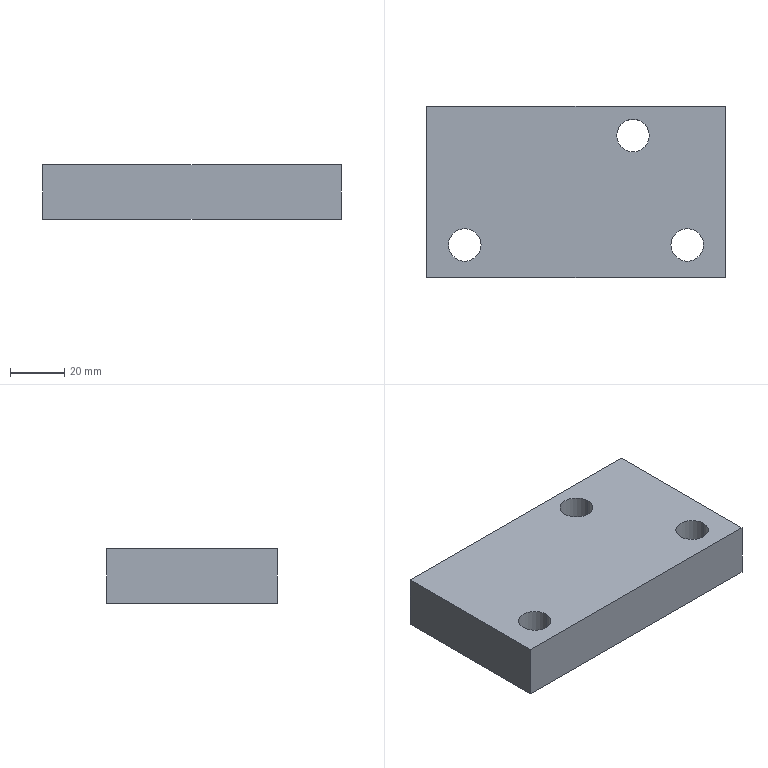Part | STEP file | cu dao nhan khong logo | 1 solid | 18 faces | box 110 x 63 x 20 mm | volume 127794 mm3 | plane 10 | cylinder 8 | commonest cylinder face diameters 12 x6 8 x2
STEP:
#1=CARTESIAN_POINT('',(0.,0.,0.));
#2=DIRECTION('',(0.,0.,1.));
#3=DIRECTION('',(1.,0.,0.));
#4=AXIS2_PLACEMENT_3D('',#1,#2,#3);
#5=CARTESIAN_POINT('',(20.,12.,0.));
#6=VERTEX_POINT('',#5);
#7=CARTESIAN_POINT('',(20.,12.,20.));
#8=VERTEX_POINT('',#7);
#9=CARTESIAN_POINT('',(20.,12.,0.));
#10=DIRECTION('',(0.,0.,1.));
#11=VECTOR('',#10,1.);
#12=LINE('',#9,#11);
#13=CARTESIAN_POINT('',(14.,12.,0.));
#14=DIRECTION('',(0.,0.,1.));
#15=DIRECTION('',(1.,0.,0.));
#16=AXIS2_PLACEMENT_3D('',#13,#14,#15);
#17=CYLINDRICAL_SURFACE('',#16,6.);
#18=CARTESIAN_POINT('',(6.283,0.));
#19=DIRECTION('',(0.,1.));
#20=VECTOR('',#19,1.);
#21=LINE('',#18,#20);
#22=(GEOMETRIC_REPRESENTATION_CONTEXT(2)PARAMETRIC_REPRESENTATION_CONTEXT()REPRESENTATION_CONTEXT('',''));
#23=DEFINITIONAL_REPRESENTATION('',(#21),#22);
#24=PCURVE('',#17,#23);
#25=CARTESIAN_POINT('',(14.,12.,0.));
#26=DIRECTION('',(0.,0.,1.));
#27=DIRECTION('',(1.,0.,0.));
#28=AXIS2_PLACEMENT_3D('',#25,#26,#27);
#29=CYLINDRICAL_SURFACE('',#28,6.);
#30=CARTESIAN_POINT('',(0.,0.));
#31=DIRECTION('',(0.,1.));
#32=VECTOR('',#31,1.);
#33=LINE('',#30,#32);
#34=(GEOMETRIC_REPRESENTATION_CONTEXT(2)PARAMETRIC_REPRESENTATION_CONTEXT()REPRESENTATION_CONTEXT('',''));
#35=DEFINITIONAL_REPRESENTATION('',(#33),#34);
#36=PCURVE('',#29,#35);
#37=SURFACE_CURVE('',#12,(#24,#36),.PCURVE_S1.);
#38=EDGE_CURVE('',#6,#8,#37,.T.);
#39=ORIENTED_EDGE('',*,*,#38,.T.);
#40=CARTESIAN_POINT('',(8.,12.,20.));
#41=VERTEX_POINT('',#40);
#42=CARTESIAN_POINT('',(14.,12.,20.));
#43=DIRECTION('',(0.,0.,-1.));
#44=DIRECTION('',(1.,0.,0.));
#45=AXIS2_PLACEMENT_3D('',#42,#43,#44);
#46=CIRCLE('',#45,6.);
#47=CARTESIAN_POINT('',(6.283,20.));
#48=DIRECTION('',(-1.,0.));
#49=VECTOR('',#48,1.);
#50=LINE('',#47,#49);
#51=(GEOMETRIC_REPRESENTATION_CONTEXT(2)PARAMETRIC_REPRESENTATION_CONTEXT()REPRESENTATION_CONTEXT('',''));
#52=DEFINITIONAL_REPRESENTATION('',(#50),#51);
#53=PCURVE('',#17,#52);
#54=CARTESIAN_POINT('',(55.,31.5,20.));
#55=DIRECTION('',(0.,0.,1.));
#56=DIRECTION('',(1.,0.,0.));
#57=AXIS2_PLACEMENT_3D('',#54,#55,#56);
#58=PLANE('',#57);
#59=CARTESIAN_POINT('',(-35.,-19.5));
#60=CARTESIAN_POINT('',(-35.,-29.892));
#61=CARTESIAN_POINT('',(-44.,-24.696));
#62=CARTESIAN_POINT('',(-53.,-19.5));
#63=CARTESIAN_POINT('',(-44.,-14.304));
#64=CARTESIAN_POINT('',(-35.,-9.108));
#65=CARTESIAN_POINT('',(-35.,-19.5));
#66=(BOUNDED_CURVE()B_SPLINE_CURVE(2,(#59,#60,#61,#62,#63,#64,#65),.UNSPECIFIED.,.T.,.F.)B_SPLINE_CURVE_WITH_KNOTS((1,2,2,2,2,1),(-2.094,0.,2.094,4.189,6.283,8.378),.UNSPECIFIED.)CURVE()GEOMETRIC_REPRESENTATION_ITEM()RATIONAL_B_SPLINE_CURVE((1.,0.5,1.,0.5,1.,0.5,1.))REPRESENTATION_ITEM(''));
#67=(GEOMETRIC_REPRESENTATION_CONTEXT(2)PARAMETRIC_REPRESENTATION_CONTEXT()REPRESENTATION_CONTEXT('',''));
#68=DEFINITIONAL_REPRESENTATION('',(#66),#67);
#69=PCURVE('',#58,#68);
#70=SURFACE_CURVE('',#46,(#53,#69),.PCURVE_S1.);
#71=EDGE_CURVE('',#8,#41,#70,.T.);
#72=ORIENTED_EDGE('',*,*,#71,.T.);
#73=CARTESIAN_POINT('',(8.,12.,0.));
#74=VERTEX_POINT('',#73);
#75=CARTESIAN_POINT('',(8.,12.,0.));
#76=DIRECTION('',(0.,0.,1.));
#77=VECTOR('',#76,1.);
#78=LINE('',#75,#77);
#79=CARTESIAN_POINT('',(3.142,0.));
#80=DIRECTION('',(0.,1.));
#81=VECTOR('',#80,1.);
#82=LINE('',#79,#81);
#83=(GEOMETRIC_REPRESENTATION_CONTEXT(2)PARAMETRIC_REPRESENTATION_CONTEXT()REPRESENTATION_CONTEXT('',''));
#84=DEFINITIONAL_REPRESENTATION('',(#82),#83);
#85=PCURVE('',#17,#84);
#86=CARTESIAN_POINT('',(3.142,0.));
#87=DIRECTION('',(0.,1.));
#88=VECTOR('',#87,1.);
#89=LINE('',#86,#88);
#90=(GEOMETRIC_REPRESENTATION_CONTEXT(2)PARAMETRIC_REPRESENTATION_CONTEXT()REPRESENTATION_CONTEXT('',''));
#91=DEFINITIONAL_REPRESENTATION('',(#89),#90);
#92=PCURVE('',#29,#91);
#93=SURFACE_CURVE('',#78,(#85,#92),.PCURVE_S1.);
#94=EDGE_CURVE('',#74,#41,#93,.T.);
#95=ORIENTED_EDGE('',*,*,#94,.F.);
#96=CARTESIAN_POINT('',(14.,12.,0.));
#97=DIRECTION('',(0.,0.,1.));
#98=DIRECTION('',(1.,0.,0.));
#99=AXIS2_PLACEMENT_3D('',#96,#97,#98);
#100=CIRCLE('',#99,6.);
#101=CARTESIAN_POINT('',(0.,0.));
#102=DIRECTION('',(1.,0.));
#103=VECTOR('',#102,1.);
#104=LINE('',#101,#103);
#105=(GEOMETRIC_REPRESENTATION_CONTEXT(2)PARAMETRIC_REPRESENTATION_CONTEXT()REPRESENTATION_CONTEXT('',''));
#106=DEFINITIONAL_REPRESENTATION('',(#104),#105);
#107=PCURVE('',#17,#106);
#108=CARTESIAN_POINT('',(55.,31.5,0.));
#109=DIRECTION('',(0.,0.,1.));
#110=DIRECTION('',(1.,0.,0.));
#111=AXIS2_PLACEMENT_3D('',#108,#109,#110);
#112=PLANE('',#111);
#113=CARTESIAN_POINT('',(-41.,-19.5));
#114=DIRECTION('',(1.,0.));
#115=AXIS2_PLACEMENT_2D('',#113,#114);
#116=CIRCLE('',#115,6.);
#117=(GEOMETRIC_REPRESENTATION_CONTEXT(2)PARAMETRIC_REPRESENTATION_CONTEXT()REPRESENTATION_CONTEXT('',''));
#118=DEFINITIONAL_REPRESENTATION('',(#116),#117);
#119=PCURVE('',#112,#118);
#120=SURFACE_CURVE('',#100,(#107,#119),.PCURVE_S1.);
#121=EDGE_CURVE('',#74,#6,#120,.T.);
#122=ORIENTED_EDGE('',*,*,#121,.T.);
#123=EDGE_LOOP('',(#39,#72,#95,#122));
#124=FACE_BOUND('',#123,.F.);
#125=ADVANCED_FACE('',(#124),#17,.F.);
#126=CARTESIAN_POINT('',(102.,12.,0.));
#127=VERTEX_POINT('',#126);
#128=CARTESIAN_POINT('',(102.,12.,20.));
#129=VERTEX_POINT('',#128);
#130=CARTESIAN_POINT('',(102.,12.,0.));
#131=DIRECTION('',(0.,0.,1.));
#132=VECTOR('',#131,1.);
#133=LINE('',#130,#132);
#134=CARTESIAN_POINT('',(96.,12.,0.));
#135=DIRECTION('',(0.,0.,1.));
#136=DIRECTION('',(1.,0.,0.));
#137=AXIS2_PLACEMENT_3D('',#134,#135,#136);
#138=CYLINDRICAL_SURFACE('',#137,6.);
#139=CARTESIAN_POINT('',(6.283,0.));
#140=DIRECTION('',(0.,1.));
#141=VECTOR('',#140,1.);
#142=LINE('',#139,#141);
#143=(GEOMETRIC_REPRESENTATION_CONTEXT(2)PARAMETRIC_REPRESENTATION_CONTEXT()REPRESENTATION_CONTEXT('',''));
#144=DEFINITIONAL_REPRESENTATION('',(#142),#143);
#145=PCURVE('',#138,#144);
#146=CARTESIAN_POINT('',(96.,12.,0.));
#147=DIRECTION('',(0.,0.,1.));
#148=DIRECTION('',(1.,0.,0.));
#149=AXIS2_PLACEMENT_3D('',#146,#147,#148);
#150=CYLINDRICAL_SURFACE('',#149,6.);
#151=CARTESIAN_POINT('',(0.,0.));
#152=DIRECTION('',(0.,1.));
#153=VECTOR('',#152,1.);
#154=LINE('',#151,#153);
#155=(GEOMETRIC_REPRESENTATION_CONTEXT(2)PARAMETRIC_REPRESENTATION_CONTEXT()REPRESENTATION_CONTEXT('',''));
#156=DEFINITIONAL_REPRESENTATION('',(#154),#155);
#157=PCURVE('',#150,#156);
#158=SURFACE_CURVE('',#133,(#145,#157),.PCURVE_S1.);
#159=EDGE_CURVE('',#127,#129,#158,.T.);
#160=ORIENTED_EDGE('',*,*,#159,.T.);
#161=CARTESIAN_POINT('',(90.,12.,20.));
#162=VERTEX_POINT('',#161);
#163=CARTESIAN_POINT('',(96.,12.,20.));
#164=DIRECTION('',(0.,0.,-1.));
#165=DIRECTION('',(1.,0.,0.));
#166=AXIS2_PLACEMENT_3D('',#163,#164,#165);
#167=CIRCLE('',#166,6.);
#168=CARTESIAN_POINT('',(6.283,20.));
#169=DIRECTION('',(-1.,0.));
#170=VECTOR('',#169,1.);
#171=LINE('',#168,#170);
#172=(GEOMETRIC_REPRESENTATION_CONTEXT(2)PARAMETRIC_REPRESENTATION_CONTEXT()REPRESENTATION_CONTEXT('',''));
#173=DEFINITIONAL_REPRESENTATION('',(#171),#172);
#174=PCURVE('',#138,#173);
#175=CARTESIAN_POINT('',(47.,-19.5));
#176=CARTESIAN_POINT('',(47.,-29.892));
#177=CARTESIAN_POINT('',(38.,-24.696));
#178=CARTESIAN_POINT('',(29.,-19.5));
#179=CARTESIAN_POINT('',(38.,-14.304));
#180=CARTESIAN_POINT('',(47.,-9.108));
#181=CARTESIAN_POINT('',(47.,-19.5));
#182=(BOUNDED_CURVE()B_SPLINE_CURVE(2,(#175,#176,#177,#178,#179,#180,#181),.UNSPECIFIED.,.T.,.F.)B_SPLINE_CURVE_WITH_KNOTS((1,2,2,2,2,1),(-2.094,0.,2.094,4.189,6.283,8.378),.UNSPECIFIED.)CURVE()GEOMETRIC_REPRESENTATION_ITEM()RATIONAL_B_SPLINE_CURVE((1.,0.5,1.,0.5,1.,0.5,1.))REPRESENTATION_ITEM(''));
#183=(GEOMETRIC_REPRESENTATION_CONTEXT(2)PARAMETRIC_REPRESENTATION_CONTEXT()REPRESENTATION_CONTEXT('',''));
#184=DEFINITIONAL_REPRESENTATION('',(#182),#183);
#185=PCURVE('',#58,#184);
#186=SURFACE_CURVE('',#167,(#174,#185),.PCURVE_S1.);
#187=EDGE_CURVE('',#129,#162,#186,.T.);
#188=ORIENTED_EDGE('',*,*,#187,.T.);
#189=CARTESIAN_POINT('',(90.,12.,0.));
#190=VERTEX_POINT('',#189);
#191=CARTESIAN_POINT('',(90.,12.,0.));
#192=DIRECTION('',(0.,0.,1.));
#193=VECTOR('',#192,1.);
#194=LINE('',#191,#193);
#195=CARTESIAN_POINT('',(3.142,0.));
#196=DIRECTION('',(0.,1.));
#197=VECTOR('',#196,1.);
#198=LINE('',#195,#197);
#199=(GEOMETRIC_REPRESENTATION_CONTEXT(2)PARAMETRIC_REPRESENTATION_CONTEXT()REPRESENTATION_CONTEXT('',''));
#200=DEFINITIONAL_REPRESENTATION('',(#198),#199);
#201=PCURVE('',#138,#200);
#202=CARTESIAN_POINT('',(3.142,0.));
#203=DIRECTION('',(0.,1.));
#204=VECTOR('',#203,1.);
#205=LINE('',#202,#204);
#206=(GEOMETRIC_REPRESENTATION_CONTEXT(2)PARAMETRIC_REPRESENTATION_CONTEXT()REPRESENTATION_CONTEXT('',''));
#207=DEFINITIONAL_REPRESENTATION('',(#205),#206);
#208=PCURVE('',#150,#207);
#209=SURFACE_CURVE('',#194,(#201,#208),.PCURVE_S1.);
#210=EDGE_CURVE('',#190,#162,#209,.T.);
#211=ORIENTED_EDGE('',*,*,#210,.F.);
#212=CARTESIAN_POINT('',(96.,12.,0.));
#213=DIRECTION('',(0.,0.,1.));
#214=DIRECTION('',(1.,0.,0.));
#215=AXIS2_PLACEMENT_3D('',#212,#213,#214);
#216=CIRCLE('',#215,6.);
#217=CARTESIAN_POINT('',(0.,0.));
#218=DIRECTION('',(1.,0.));
#219=VECTOR('',#218,1.);
#220=LINE('',#217,#219);
#221=(GEOMETRIC_REPRESENTATION_CONTEXT(2)PARAMETRIC_REPRESENTATION_CONTEXT()REPRESENTATION_CONTEXT('',''));
#222=DEFINITIONAL_REPRESENTATION('',(#220),#221);
#223=PCURVE('',#138,#222);
#224=CARTESIAN_POINT('',(41.,-19.5));
#225=DIRECTION('',(1.,0.));
#226=AXIS2_PLACEMENT_2D('',#224,#225);
#227=CIRCLE('',#226,6.);
#228=(GEOMETRIC_REPRESENTATION_CONTEXT(2)PARAMETRIC_REPRESENTATION_CONTEXT()REPRESENTATION_CONTEXT('',''));
#229=DEFINITIONAL_REPRESENTATION('',(#227),#228);
#230=PCURVE('',#112,#229);
#231=SURFACE_CURVE('',#216,(#223,#230),.PCURVE_S1.);
#232=EDGE_CURVE('',#190,#127,#231,.T.);
#233=ORIENTED_EDGE('',*,*,#232,.T.);
#234=EDGE_LOOP('',(#160,#188,#211,#233));
#235=FACE_BOUND('',#234,.F.);
#236=ADVANCED_FACE('',(#235),#138,.F.);
#237=CARTESIAN_POINT('',(82.,52.3,5.));
#238=VERTEX_POINT('',#237);
#239=CARTESIAN_POINT('',(82.,52.3,20.));
#240=VERTEX_POINT('',#239);
#241=CARTESIAN_POINT('',(82.,52.3,5.));
#242=DIRECTION('',(0.,0.,1.));
#243=VECTOR('',#242,1.);
#244=LINE('',#241,#243);
#245=CARTESIAN_POINT('',(76.,52.3,5.));
#246=DIRECTION('',(0.,0.,1.));
#247=DIRECTION('',(1.,0.,0.));
#248=AXIS2_PLACEMENT_3D('',#245,#246,#247);
#249=CYLINDRICAL_SURFACE('',#248,6.);
#250=CARTESIAN_POINT('',(6.283,0.));
#251=DIRECTION('',(0.,1.));
#252=VECTOR('',#251,1.);
#253=LINE('',#250,#252);
#254=(GEOMETRIC_REPRESENTATION_CONTEXT(2)PARAMETRIC_REPRESENTATION_CONTEXT()REPRESENTATION_CONTEXT('',''));
#255=DEFINITIONAL_REPRESENTATION('',(#253),#254);
#256=PCURVE('',#249,#255);
#257=CARTESIAN_POINT('',(76.,52.3,5.));
#258=DIRECTION('',(0.,0.,1.));
#259=DIRECTION('',(1.,0.,0.));
#260=AXIS2_PLACEMENT_3D('',#257,#258,#259);
#261=CYLINDRICAL_SURFACE('',#260,6.);
#262=CARTESIAN_POINT('',(0.,0.));
#263=DIRECTION('',(0.,1.));
#264=VECTOR('',#263,1.);
#265=LINE('',#262,#264);
#266=(GEOMETRIC_REPRESENTATION_CONTEXT(2)PARAMETRIC_REPRESENTATION_CONTEXT()REPRESENTATION_CONTEXT('',''));
#267=DEFINITIONAL_REPRESENTATION('',(#265),#266);
#268=PCURVE('',#261,#267);
#269=SURFACE_CURVE('',#244,(#256,#268),.PCURVE_S1.);
#270=EDGE_CURVE('',#238,#240,#269,.T.);
#271=ORIENTED_EDGE('',*,*,#270,.T.);
#272=CARTESIAN_POINT('',(70.,52.3,20.));
#273=VERTEX_POINT('',#272);
#274=CARTESIAN_POINT('',(76.,52.3,20.));
#275=DIRECTION('',(0.,0.,-1.));
#276=DIRECTION('',(1.,0.,0.));
#277=AXIS2_PLACEMENT_3D('',#274,#275,#276);
#278=CIRCLE('',#277,6.);
#279=CARTESIAN_POINT('',(6.283,15.));
#280=DIRECTION('',(-1.,0.));
#281=VECTOR('',#280,1.);
#282=LINE('',#279,#281);
#283=(GEOMETRIC_REPRESENTATION_CONTEXT(2)PARAMETRIC_REPRESENTATION_CONTEXT()REPRESENTATION_CONTEXT('',''));
#284=DEFINITIONAL_REPRESENTATION('',(#282),#283);
#285=PCURVE('',#249,#284);
#286=CARTESIAN_POINT('',(27.,20.8));
#287=CARTESIAN_POINT('',(27.,10.408));
#288=CARTESIAN_POINT('',(18.,15.604));
#289=CARTESIAN_POINT('',(9.,20.8));
#290=CARTESIAN_POINT('',(18.,25.996));
#291=CARTESIAN_POINT('',(27.,31.192));
#292=CARTESIAN_POINT('',(27.,20.8));
#293=(BOUNDED_CURVE()B_SPLINE_CURVE(2,(#286,#287,#288,#289,#290,#291,#292),.UNSPECIFIED.,.T.,.F.)B_SPLINE_CURVE_WITH_KNOTS((1,2,2,2,2,1),(-2.094,0.,2.094,4.189,6.283,8.378),.UNSPECIFIED.)CURVE()GEOMETRIC_REPRESENTATION_ITEM()RATIONAL_B_SPLINE_CURVE((1.,0.5,1.,0.5,1.,0.5,1.))REPRESENTATION_ITEM(''));
#294=(GEOMETRIC_REPRESENTATION_CONTEXT(2)PARAMETRIC_REPRESENTATION_CONTEXT()REPRESENTATION_CONTEXT('',''));
#295=DEFINITIONAL_REPRESENTATION('',(#293),#294);
#296=PCURVE('',#58,#295);
#297=SURFACE_CURVE('',#278,(#285,#296),.PCURVE_S1.);
#298=EDGE_CURVE('',#240,#273,#297,.T.);
#299=ORIENTED_EDGE('',*,*,#298,.T.);
#300=CARTESIAN_POINT('',(70.,52.3,5.));
#301=VERTEX_POINT('',#300);
#302=CARTESIAN_POINT('',(70.,52.3,5.));
#303=DIRECTION('',(0.,0.,1.));
#304=VECTOR('',#303,1.);
#305=LINE('',#302,#304);
#306=CARTESIAN_POINT('',(3.142,0.));
#307=DIRECTION('',(0.,1.));
#308=VECTOR('',#307,1.);
#309=LINE('',#306,#308);
#310=(GEOMETRIC_REPRESENTATION_CONTEXT(2)PARAMETRIC_REPRESENTATION_CONTEXT()REPRESENTATION_CONTEXT('',''));
#311=DEFINITIONAL_REPRESENTATION('',(#309),#310);
#312=PCURVE('',#249,#311);
#313=CARTESIAN_POINT('',(3.142,0.));
#314=DIRECTION('',(0.,1.));
#315=VECTOR('',#314,1.);
#316=LINE('',#313,#315);
#317=(GEOMETRIC_REPRESENTATION_CONTEXT(2)PARAMETRIC_REPRESENTATION_CONTEXT()REPRESENTATION_CONTEXT('',''));
#318=DEFINITIONAL_REPRESENTATION('',(#316),#317);
#319=PCURVE('',#261,#318);
#320=SURFACE_CURVE('',#305,(#312,#319),.PCURVE_S1.);
#321=EDGE_CURVE('',#301,#273,#320,.T.);
#322=ORIENTED_EDGE('',*,*,#321,.F.);
#323=CARTESIAN_POINT('',(76.,52.3,5.));
#324=DIRECTION('',(0.,0.,1.));
#325=DIRECTION('',(1.,0.,0.));
#326=AXIS2_PLACEMENT_3D('',#323,#324,#325);
#327=CIRCLE('',#326,6.);
#328=CARTESIAN_POINT('',(0.,0.));
#329=DIRECTION('',(1.,0.));
#330=VECTOR('',#329,1.);
#331=LINE('',#328,#330);
#332=(GEOMETRIC_REPRESENTATION_CONTEXT(2)PARAMETRIC_REPRESENTATION_CONTEXT()REPRESENTATION_CONTEXT('',''));
#333=DEFINITIONAL_REPRESENTATION('',(#331),#332);
#334=PCURVE('',#249,#333);
#335=CARTESIAN_POINT('',(76.,52.327,5.));
#336=DIRECTION('',(0.,0.,1.));
#337=DIRECTION('',(1.,0.,0.));
#338=AXIS2_PLACEMENT_3D('',#335,#336,#337);
#339=PLANE('',#338);
#340=CARTESIAN_POINT('',(0.,-0.02689));
#341=DIRECTION('',(1.,0.));
#342=AXIS2_PLACEMENT_2D('',#340,#341);
#343=CIRCLE('',#342,6.);
#344=(GEOMETRIC_REPRESENTATION_CONTEXT(2)PARAMETRIC_REPRESENTATION_CONTEXT()REPRESENTATION_CONTEXT('',''));
#345=DEFINITIONAL_REPRESENTATION('',(#343),#344);
#346=PCURVE('',#339,#345);
#347=SURFACE_CURVE('',#327,(#334,#346),.PCURVE_S1.);
#348=EDGE_CURVE('',#301,#238,#347,.T.);
#349=ORIENTED_EDGE('',*,*,#348,.T.);
#350=EDGE_LOOP('',(#271,#299,#322,#349));
#351=FACE_BOUND('',#350,.F.);
#352=ADVANCED_FACE('',(#351),#249,.F.);
#353=ORIENTED_EDGE('',*,*,#71,.T.);
#354=CARTESIAN_POINT('',(14.,12.,20.));
#355=DIRECTION('',(0.,0.,-1.));
#356=DIRECTION('',(1.,0.,0.));
#357=AXIS2_PLACEMENT_3D('',#354,#355,#356);
#358=CIRCLE('',#357,6.);
#359=CARTESIAN_POINT('',(-35.,-19.5));
#360=CARTESIAN_POINT('',(-35.,-29.892));
#361=CARTESIAN_POINT('',(-44.,-24.696));
#362=CARTESIAN_POINT('',(-53.,-19.5));
#363=CARTESIAN_POINT('',(-44.,-14.304));
#364=CARTESIAN_POINT('',(-35.,-9.108));
#365=CARTESIAN_POINT('',(-35.,-19.5));
#366=(BOUNDED_CURVE()B_SPLINE_CURVE(2,(#359,#360,#361,#362,#363,#364,#365),.UNSPECIFIED.,.T.,.F.)B_SPLINE_CURVE_WITH_KNOTS((1,2,2,2,2,1),(-2.094,0.,2.094,4.189,6.283,8.378),.UNSPECIFIED.)CURVE()GEOMETRIC_REPRESENTATION_ITEM()RATIONAL_B_SPLINE_CURVE((1.,0.5,1.,0.5,1.,0.5,1.))REPRESENTATION_ITEM(''));
#367=(GEOMETRIC_REPRESENTATION_CONTEXT(2)PARAMETRIC_REPRESENTATION_CONTEXT()REPRESENTATION_CONTEXT('',''));
#368=DEFINITIONAL_REPRESENTATION('',(#366),#367);
#369=PCURVE('',#58,#368);
#370=CARTESIAN_POINT('',(6.283,20.));
#371=DIRECTION('',(-1.,0.));
#372=VECTOR('',#371,1.);
#373=LINE('',#370,#372);
#374=(GEOMETRIC_REPRESENTATION_CONTEXT(2)PARAMETRIC_REPRESENTATION_CONTEXT()REPRESENTATION_CONTEXT('',''));
#375=DEFINITIONAL_REPRESENTATION('',(#373),#374);
#376=PCURVE('',#29,#375);
#377=SURFACE_CURVE('',#358,(#369,#376),.PCURVE_S1.);
#378=EDGE_CURVE('',#41,#8,#377,.T.);
#379=ORIENTED_EDGE('',*,*,#378,.T.);
#380=EDGE_LOOP('',(#353,#379));
#381=FACE_BOUND('',#380,.T.);
#382=ORIENTED_EDGE('',*,*,#187,.T.);
#383=CARTESIAN_POINT('',(96.,12.,20.));
#384=DIRECTION('',(0.,0.,-1.));
#385=DIRECTION('',(1.,0.,0.));
#386=AXIS2_PLACEMENT_3D('',#383,#384,#385);
#387=CIRCLE('',#386,6.);
#388=CARTESIAN_POINT('',(47.,-19.5));
#389=CARTESIAN_POINT('',(47.,-29.892));
#390=CARTESIAN_POINT('',(38.,-24.696));
#391=CARTESIAN_POINT('',(29.,-19.5));
#392=CARTESIAN_POINT('',(38.,-14.304));
#393=CARTESIAN_POINT('',(47.,-9.108));
#394=CARTESIAN_POINT('',(47.,-19.5));
#395=(BOUNDED_CURVE()B_SPLINE_CURVE(2,(#388,#389,#390,#391,#392,#393,#394),.UNSPECIFIED.,.T.,.F.)B_SPLINE_CURVE_WITH_KNOTS((1,2,2,2,2,1),(-2.094,0.,2.094,4.189,6.283,8.378),.UNSPECIFIED.)CURVE()GEOMETRIC_REPRESENTATION_ITEM()RATIONAL_B_SPLINE_CURVE((1.,0.5,1.,0.5,1.,0.5,1.))REPRESENTATION_ITEM(''));
#396=(GEOMETRIC_REPRESENTATION_CONTEXT(2)PARAMETRIC_REPRESENTATION_CONTEXT()REPRESENTATION_CONTEXT('',''));
#397=DEFINITIONAL_REPRESENTATION('',(#395),#396);
#398=PCURVE('',#58,#397);
#399=CARTESIAN_POINT('',(6.283,20.));
#400=DIRECTION('',(-1.,0.));
#401=VECTOR('',#400,1.);
#402=LINE('',#399,#401);
#403=(GEOMETRIC_REPRESENTATION_CONTEXT(2)PARAMETRIC_REPRESENTATION_CONTEXT()REPRESENTATION_CONTEXT('',''));
#404=DEFINITIONAL_REPRESENTATION('',(#402),#403);
#405=PCURVE('',#150,#404);
#406=SURFACE_CURVE('',#387,(#398,#405),.PCURVE_S1.);
#407=EDGE_CURVE('',#162,#129,#406,.T.);
#408=ORIENTED_EDGE('',*,*,#407,.T.);
#409=EDGE_LOOP('',(#382,#408));
#410=FACE_BOUND('',#409,.T.);
#411=ORIENTED_EDGE('',*,*,#298,.T.);
#412=CARTESIAN_POINT('',(76.,52.3,20.));
#413=DIRECTION('',(0.,0.,-1.));
#414=DIRECTION('',(1.,0.,0.));
#415=AXIS2_PLACEMENT_3D('',#412,#413,#414);
#416=CIRCLE('',#415,6.);
#417=CARTESIAN_POINT('',(27.,20.8));
#418=CARTESIAN_POINT('',(27.,10.408));
#419=CARTESIAN_POINT('',(18.,15.604));
#420=CARTESIAN_POINT('',(9.,20.8));
#421=CARTESIAN_POINT('',(18.,25.996));
#422=CARTESIAN_POINT('',(27.,31.192));
#423=CARTESIAN_POINT('',(27.,20.8));
#424=(BOUNDED_CURVE()B_SPLINE_CURVE(2,(#417,#418,#419,#420,#421,#422,#423),.UNSPECIFIED.,.T.,.F.)B_SPLINE_CURVE_WITH_KNOTS((1,2,2,2,2,1),(-2.094,0.,2.094,4.189,6.283,8.378),.UNSPECIFIED.)CURVE()GEOMETRIC_REPRESENTATION_ITEM()RATIONAL_B_SPLINE_CURVE((1.,0.5,1.,0.5,1.,0.5,1.))REPRESENTATION_ITEM(''));
#425=(GEOMETRIC_REPRESENTATION_CONTEXT(2)PARAMETRIC_REPRESENTATION_CONTEXT()REPRESENTATION_CONTEXT('',''));
#426=DEFINITIONAL_REPRESENTATION('',(#424),#425);
#427=PCURVE('',#58,#426);
#428=CARTESIAN_POINT('',(6.283,15.));
#429=DIRECTION('',(-1.,0.));
#430=VECTOR('',#429,1.);
#431=LINE('',#428,#430);
#432=(GEOMETRIC_REPRESENTATION_CONTEXT(2)PARAMETRIC_REPRESENTATION_CONTEXT()REPRESENTATION_CONTEXT('',''));
#433=DEFINITIONAL_REPRESENTATION('',(#431),#432);
#434=PCURVE('',#261,#433);
#435=SURFACE_CURVE('',#416,(#427,#434),.PCURVE_S1.);
#436=EDGE_CURVE('',#273,#240,#435,.T.);
#437=ORIENTED_EDGE('',*,*,#436,.T.);
#438=EDGE_LOOP('',(#411,#437));
#439=FACE_BOUND('',#438,.T.);
#440=CARTESIAN_POINT('',(110.,0.,20.));
#441=VERTEX_POINT('',#440);
#442=CARTESIAN_POINT('',(110.,63.,20.));
#443=VERTEX_POINT('',#442);
#444=CARTESIAN_POINT('',(110.,31.5,20.));
#445=DIRECTION('',(0.,1.,0.));
#446=VECTOR('',#445,1.);
#447=LINE('',#444,#446);
#448=CARTESIAN_POINT('',(55.,0.));
#449=DIRECTION('',(0.,1.));
#450=VECTOR('',#449,1.);
#451=LINE('',#448,#450);
#452=(GEOMETRIC_REPRESENTATION_CONTEXT(2)PARAMETRIC_REPRESENTATION_CONTEXT()REPRESENTATION_CONTEXT('',''));
#453=DEFINITIONAL_REPRESENTATION('',(#451),#452);
#454=PCURVE('',#58,#453);
#455=CARTESIAN_POINT('',(110.,63.,0.));
#456=DIRECTION('',(1.,0.,0.));
#457=DIRECTION('',(0.,0.,-1.));
#458=AXIS2_PLACEMENT_3D('',#455,#456,#457);
#459=PLANE('',#458);
#460=CARTESIAN_POINT('',(-20.,-31.5));
#461=DIRECTION('',(0.,1.));
#462=VECTOR('',#461,1.);
#463=LINE('',#460,#462);
#464=(GEOMETRIC_REPRESENTATION_CONTEXT(2)PARAMETRIC_REPRESENTATION_CONTEXT()REPRESENTATION_CONTEXT('',''));
#465=DEFINITIONAL_REPRESENTATION('',(#463),#464);
#466=PCURVE('',#459,#465);
#467=SURFACE_CURVE('',#447,(#454,#466),.PCURVE_S1.);
#468=EDGE_CURVE('',#441,#443,#467,.T.);
#469=ORIENTED_EDGE('',*,*,#468,.T.);
#470=CARTESIAN_POINT('',(0.,63.,20.));
#471=VERTEX_POINT('',#470);
#472=CARTESIAN_POINT('',(55.,63.,20.));
#473=DIRECTION('',(-1.,0.,0.));
#474=VECTOR('',#473,1.);
#475=LINE('',#472,#474);
#476=CARTESIAN_POINT('',(0.,31.5));
#477=DIRECTION('',(-1.,0.));
#478=VECTOR('',#477,1.);
#479=LINE('',#476,#478);
#480=(GEOMETRIC_REPRESENTATION_CONTEXT(2)PARAMETRIC_REPRESENTATION_CONTEXT()REPRESENTATION_CONTEXT('',''));
#481=DEFINITIONAL_REPRESENTATION('',(#479),#480);
#482=PCURVE('',#58,#481);
#483=CARTESIAN_POINT('',(0.,63.,0.));
#484=DIRECTION('',(0.,1.,0.));
#485=DIRECTION('',(0.,0.,1.));
#486=AXIS2_PLACEMENT_3D('',#483,#484,#485);
#487=PLANE('',#486);
#488=CARTESIAN_POINT('',(20.,55.));
#489=DIRECTION('',(0.,-1.));
#490=VECTOR('',#489,1.);
#491=LINE('',#488,#490);
#492=(GEOMETRIC_REPRESENTATION_CONTEXT(2)PARAMETRIC_REPRESENTATION_CONTEXT()REPRESENTATION_CONTEXT('',''));
#493=DEFINITIONAL_REPRESENTATION('',(#491),#492);
#494=PCURVE('',#487,#493);
#495=SURFACE_CURVE('',#475,(#482,#494),.PCURVE_S1.);
#496=EDGE_CURVE('',#443,#471,#495,.T.);
#497=ORIENTED_EDGE('',*,*,#496,.T.);
#498=CARTESIAN_POINT('',(0.,0.,20.));
#499=VERTEX_POINT('',#498);
#500=CARTESIAN_POINT('',(0.,31.5,20.));
#501=DIRECTION('',(0.,-1.,0.));
#502=VECTOR('',#501,1.);
#503=LINE('',#500,#502);
#504=CARTESIAN_POINT('',(-55.,0.));
#505=DIRECTION('',(0.,-1.));
#506=VECTOR('',#505,1.);
#507=LINE('',#504,#506);
#508=(GEOMETRIC_REPRESENTATION_CONTEXT(2)PARAMETRIC_REPRESENTATION_CONTEXT()REPRESENTATION_CONTEXT('',''));
#509=DEFINITIONAL_REPRESENTATION('',(#507),#508);
#510=PCURVE('',#58,#509);
#511=CARTESIAN_POINT('',(0.,0.,0.));
#512=DIRECTION('',(-1.,0.,0.));
#513=DIRECTION('',(0.,0.,1.));
#514=AXIS2_PLACEMENT_3D('',#511,#512,#513);
#515=PLANE('',#514);
#516=CARTESIAN_POINT('',(20.,31.5));
#517=DIRECTION('',(0.,-1.));
#518=VECTOR('',#517,1.);
#519=LINE('',#516,#518);
#520=(GEOMETRIC_REPRESENTATION_CONTEXT(2)PARAMETRIC_REPRESENTATION_CONTEXT()REPRESENTATION_CONTEXT('',''));
#521=DEFINITIONAL_REPRESENTATION('',(#519),#520);
#522=PCURVE('',#515,#521);
#523=SURFACE_CURVE('',#503,(#510,#522),.PCURVE_S1.);
#524=EDGE_CURVE('',#471,#499,#523,.T.);
#525=ORIENTED_EDGE('',*,*,#524,.T.);
#526=CARTESIAN_POINT('',(55.,0.,20.));
#527=DIRECTION('',(1.,0.,0.));
#528=VECTOR('',#527,1.);
#529=LINE('',#526,#528);
#530=CARTESIAN_POINT('',(0.,-31.5));
#531=DIRECTION('',(1.,0.));
#532=VECTOR('',#531,1.);
#533=LINE('',#530,#532);
#534=(GEOMETRIC_REPRESENTATION_CONTEXT(2)PARAMETRIC_REPRESENTATION_CONTEXT()REPRESENTATION_CONTEXT('',''));
#535=DEFINITIONAL_REPRESENTATION('',(#533),#534);
#536=PCURVE('',#58,#535);
#537=CARTESIAN_POINT('',(110.,0.,0.));
#538=DIRECTION('',(0.,-1.,0.));
#539=DIRECTION('',(0.,0.,-1.));
#540=AXIS2_PLACEMENT_3D('',#537,#538,#539);
#541=PLANE('',#540);
#542=CARTESIAN_POINT('',(-20.,-55.));
#543=DIRECTION('',(0.,1.));
#544=VECTOR('',#543,1.);
#545=LINE('',#542,#544);
#546=(GEOMETRIC_REPRESENTATION_CONTEXT(2)PARAMETRIC_REPRESENTATION_CONTEXT()REPRESENTATION_CONTEXT('',''));
#547=DEFINITIONAL_REPRESENTATION('',(#545),#546);
#548=PCURVE('',#541,#547);
#549=SURFACE_CURVE('',#529,(#536,#548),.PCURVE_S1.);
#550=EDGE_CURVE('',#499,#441,#549,.T.);
#551=ORIENTED_EDGE('',*,*,#550,.T.);
#552=EDGE_LOOP('',(#469,#497,#525,#551));
#553=FACE_BOUND('',#552,.T.);
#554=ADVANCED_FACE('',(#381,#410,#439,#553),#58,.T.);
#555=ORIENTED_EDGE('',*,*,#378,.T.);
#556=ORIENTED_EDGE('',*,*,#38,.F.);
#557=CARTESIAN_POINT('',(14.,12.,0.));
#558=DIRECTION('',(0.,0.,1.));
#559=DIRECTION('',(1.,0.,0.));
#560=AXIS2_PLACEMENT_3D('',#557,#558,#559);
#561=CIRCLE('',#560,6.);
#562=CARTESIAN_POINT('',(0.,0.));
#563=DIRECTION('',(1.,0.));
#564=VECTOR('',#563,1.);
#565=LINE('',#562,#564);
#566=(GEOMETRIC_REPRESENTATION_CONTEXT(2)PARAMETRIC_REPRESENTATION_CONTEXT()REPRESENTATION_CONTEXT('',''));
#567=DEFINITIONAL_REPRESENTATION('',(#565),#566);
#568=PCURVE('',#29,#567);
#569=CARTESIAN_POINT('',(-41.,-19.5));
#570=DIRECTION('',(1.,0.));
#571=AXIS2_PLACEMENT_2D('',#569,#570);
#572=CIRCLE('',#571,6.);
#573=(GEOMETRIC_REPRESENTATION_CONTEXT(2)PARAMETRIC_REPRESENTATION_CONTEXT()REPRESENTATION_CONTEXT('',''));
#574=DEFINITIONAL_REPRESENTATION('',(#572),#573);
#575=PCURVE('',#112,#574);
#576=SURFACE_CURVE('',#561,(#568,#575),.PCURVE_S1.);
#577=EDGE_CURVE('',#6,#74,#576,.T.);
#578=ORIENTED_EDGE('',*,*,#577,.T.);
#579=ORIENTED_EDGE('',*,*,#94,.T.);
#580=EDGE_LOOP('',(#555,#556,#578,#579));
#581=FACE_BOUND('',#580,.F.);
#582=ADVANCED_FACE('',(#581),#29,.F.);
#583=ORIENTED_EDGE('',*,*,#407,.T.);
#584=ORIENTED_EDGE('',*,*,#159,.F.);
#585=CARTESIAN_POINT('',(96.,12.,0.));
#586=DIRECTION('',(0.,0.,1.));
#587=DIRECTION('',(1.,0.,0.));
#588=AXIS2_PLACEMENT_3D('',#585,#586,#587);
#589=CIRCLE('',#588,6.);
#590=CARTESIAN_POINT('',(0.,0.));
#591=DIRECTION('',(1.,0.));
#592=VECTOR('',#591,1.);
#593=LINE('',#590,#592);
#594=(GEOMETRIC_REPRESENTATION_CONTEXT(2)PARAMETRIC_REPRESENTATION_CONTEXT()REPRESENTATION_CONTEXT('',''));
#595=DEFINITIONAL_REPRESENTATION('',(#593),#594);
#596=PCURVE('',#150,#595);
#597=CARTESIAN_POINT('',(41.,-19.5));
#598=DIRECTION('',(1.,0.));
#599=AXIS2_PLACEMENT_2D('',#597,#598);
#600=CIRCLE('',#599,6.);
#601=(GEOMETRIC_REPRESENTATION_CONTEXT(2)PARAMETRIC_REPRESENTATION_CONTEXT()REPRESENTATION_CONTEXT('',''));
#602=DEFINITIONAL_REPRESENTATION('',(#600),#601);
#603=PCURVE('',#112,#602);
#604=SURFACE_CURVE('',#589,(#596,#603),.PCURVE_S1.);
#605=EDGE_CURVE('',#127,#190,#604,.T.);
#606=ORIENTED_EDGE('',*,*,#605,.T.);
#607=ORIENTED_EDGE('',*,*,#210,.T.);
#608=EDGE_LOOP('',(#583,#584,#606,#607));
#609=FACE_BOUND('',#608,.F.);
#610=ADVANCED_FACE('',(#609),#150,.F.);
#611=ORIENTED_EDGE('',*,*,#436,.T.);
#612=ORIENTED_EDGE('',*,*,#270,.F.);
#613=CARTESIAN_POINT('',(76.,52.3,5.));
#614=DIRECTION('',(0.,0.,1.));
#615=DIRECTION('',(1.,0.,0.));
#616=AXIS2_PLACEMENT_3D('',#613,#614,#615);
#617=CIRCLE('',#616,6.);
#618=CARTESIAN_POINT('',(0.,0.));
#619=DIRECTION('',(1.,0.));
#620=VECTOR('',#619,1.);
#621=LINE('',#618,#620);
#622=(GEOMETRIC_REPRESENTATION_CONTEXT(2)PARAMETRIC_REPRESENTATION_CONTEXT()REPRESENTATION_CONTEXT('',''));
#623=DEFINITIONAL_REPRESENTATION('',(#621),#622);
#624=PCURVE('',#261,#623);
#625=CARTESIAN_POINT('',(0.,-0.02689));
#626=DIRECTION('',(1.,0.));
#627=AXIS2_PLACEMENT_2D('',#625,#626);
#628=CIRCLE('',#627,6.);
#629=(GEOMETRIC_REPRESENTATION_CONTEXT(2)PARAMETRIC_REPRESENTATION_CONTEXT()REPRESENTATION_CONTEXT('',''));
#630=DEFINITIONAL_REPRESENTATION('',(#628),#629);
#631=PCURVE('',#339,#630);
#632=SURFACE_CURVE('',#617,(#624,#631),.PCURVE_S1.);
#633=EDGE_CURVE('',#238,#301,#632,.T.);
#634=ORIENTED_EDGE('',*,*,#633,.T.);
#635=ORIENTED_EDGE('',*,*,#321,.T.);
#636=EDGE_LOOP('',(#611,#612,#634,#635));
#637=FACE_BOUND('',#636,.F.);
#638=ADVANCED_FACE('',(#637),#261,.F.);
#639=CARTESIAN_POINT('',(110.,63.,0.));
#640=VERTEX_POINT('',#639);
#641=CARTESIAN_POINT('',(110.,63.,0.));
#642=DIRECTION('',(0.,0.,-1.));
#643=VECTOR('',#642,1.);
#644=LINE('',#641,#643);
#645=CARTESIAN_POINT('',(0.,110.));
#646=DIRECTION('',(-1.,0.));
#647=VECTOR('',#646,1.);
#648=LINE('',#645,#647);
#649=(GEOMETRIC_REPRESENTATION_CONTEXT(2)PARAMETRIC_REPRESENTATION_CONTEXT()REPRESENTATION_CONTEXT('',''));
#650=DEFINITIONAL_REPRESENTATION('',(#648),#649);
#651=PCURVE('',#487,#650);
#652=CARTESIAN_POINT('',(0.,0.));
#653=DIRECTION('',(1.,0.));
#654=VECTOR('',#653,1.);
#655=LINE('',#652,#654);
#656=(GEOMETRIC_REPRESENTATION_CONTEXT(2)PARAMETRIC_REPRESENTATION_CONTEXT()REPRESENTATION_CONTEXT('',''));
#657=DEFINITIONAL_REPRESENTATION('',(#655),#656);
#658=PCURVE('',#459,#657);
#659=SURFACE_CURVE('',#644,(#651,#658),.PCURVE_S1.);
#660=EDGE_CURVE('',#443,#640,#659,.T.);
#661=ORIENTED_EDGE('',*,*,#660,.T.);
#662=CARTESIAN_POINT('',(97.,63.,0.));
#663=VERTEX_POINT('',#662);
#664=CARTESIAN_POINT('',(0.,63.,0.));
#665=DIRECTION('',(-1.,0.,0.));
#666=VECTOR('',#665,1.);
#667=LINE('',#664,#666);
#668=CARTESIAN_POINT('',(0.,0.));
#669=DIRECTION('',(0.,-1.));
#670=VECTOR('',#669,1.);
#671=LINE('',#668,#670);
#672=(GEOMETRIC_REPRESENTATION_CONTEXT(2)PARAMETRIC_REPRESENTATION_CONTEXT()REPRESENTATION_CONTEXT('',''));
#673=DEFINITIONAL_REPRESENTATION('',(#671),#672);
#674=PCURVE('',#487,#673);
#675=CARTESIAN_POINT('',(-55.,31.5));
#676=DIRECTION('',(-1.,0.));
#677=VECTOR('',#676,1.);
#678=LINE('',#675,#677);
#679=(GEOMETRIC_REPRESENTATION_CONTEXT(2)PARAMETRIC_REPRESENTATION_CONTEXT()REPRESENTATION_CONTEXT('',''));
#680=DEFINITIONAL_REPRESENTATION('',(#678),#679);
#681=PCURVE('',#112,#680);
#682=SURFACE_CURVE('',#667,(#674,#681),.PCURVE_S1.);
#683=EDGE_CURVE('',#640,#663,#682,.T.);
#684=ORIENTED_EDGE('',*,*,#683,.T.);
#685=CARTESIAN_POINT('',(97.,63.,5.));
#686=VERTEX_POINT('',#685);
#687=CARTESIAN_POINT('',(97.,63.,0.));
#688=DIRECTION('',(0.,0.,1.));
#689=VECTOR('',#688,1.);
#690=LINE('',#687,#689);
#691=CARTESIAN_POINT('',(0.,97.));
#692=DIRECTION('',(1.,0.));
#693=VECTOR('',#692,1.);
#694=LINE('',#691,#693);
#695=(GEOMETRIC_REPRESENTATION_CONTEXT(2)PARAMETRIC_REPRESENTATION_CONTEXT()REPRESENTATION_CONTEXT('',''));
#696=DEFINITIONAL_REPRESENTATION('',(#694),#695);
#697=PCURVE('',#487,#696);
#698=CARTESIAN_POINT('',(97.,63.,0.));
#699=DIRECTION('',(1.,0.,0.));
#700=DIRECTION('',(0.,0.,-1.));
#701=AXIS2_PLACEMENT_3D('',#698,#699,#700);
#702=PLANE('',#701);
#703=CARTESIAN_POINT('',(0.,0.));
#704=DIRECTION('',(-1.,0.));
#705=VECTOR('',#704,1.);
#706=LINE('',#703,#705);
#707=(GEOMETRIC_REPRESENTATION_CONTEXT(2)PARAMETRIC_REPRESENTATION_CONTEXT()REPRESENTATION_CONTEXT('',''));
#708=DEFINITIONAL_REPRESENTATION('',(#706),#707);
#709=PCURVE('',#702,#708);
#710=SURFACE_CURVE('',#690,(#697,#709),.PCURVE_S1.);
#711=EDGE_CURVE('',#663,#686,#710,.T.);
#712=ORIENTED_EDGE('',*,*,#711,.T.);
#713=CARTESIAN_POINT('',(55.,63.,5.));
#714=VERTEX_POINT('',#713);
#715=CARTESIAN_POINT('',(0.,63.,5.));
#716=DIRECTION('',(-1.,0.,0.));
#717=VECTOR('',#716,1.);
#718=LINE('',#715,#717);
#719=CARTESIAN_POINT('',(5.,0.));
#720=DIRECTION('',(0.,-1.));
#721=VECTOR('',#720,1.);
#722=LINE('',#719,#721);
#723=(GEOMETRIC_REPRESENTATION_CONTEXT(2)PARAMETRIC_REPRESENTATION_CONTEXT()REPRESENTATION_CONTEXT('',''));
#724=DEFINITIONAL_REPRESENTATION('',(#722),#723);
#725=PCURVE('',#487,#724);
#726=CARTESIAN_POINT('',(-76.,10.673));
#727=DIRECTION('',(-1.,0.));
#728=VECTOR('',#727,1.);
#729=LINE('',#726,#728);
#730=(GEOMETRIC_REPRESENTATION_CONTEXT(2)PARAMETRIC_REPRESENTATION_CONTEXT()REPRESENTATION_CONTEXT('',''));
#731=DEFINITIONAL_REPRESENTATION('',(#729),#730);
#732=PCURVE('',#339,#731);
#733=SURFACE_CURVE('',#718,(#725,#732),.PCURVE_S1.);
#734=EDGE_CURVE('',#686,#714,#733,.T.);
#735=ORIENTED_EDGE('',*,*,#734,.T.);
#736=CARTESIAN_POINT('',(55.,63.,0.));
#737=VERTEX_POINT('',#736);
#738=CARTESIAN_POINT('',(55.,63.,0.));
#739=DIRECTION('',(0.,0.,-1.));
#740=VECTOR('',#739,1.);
#741=LINE('',#738,#740);
#742=CARTESIAN_POINT('',(0.,55.));
#743=DIRECTION('',(-1.,0.));
#744=VECTOR('',#743,1.);
#745=LINE('',#742,#744);
#746=(GEOMETRIC_REPRESENTATION_CONTEXT(2)PARAMETRIC_REPRESENTATION_CONTEXT()REPRESENTATION_CONTEXT('',''));
#747=DEFINITIONAL_REPRESENTATION('',(#745),#746);
#748=PCURVE('',#487,#747);
#749=CARTESIAN_POINT('',(55.,45.,0.));
#750=DIRECTION('',(-1.,0.,0.));
#751=DIRECTION('',(0.,0.,1.));
#752=AXIS2_PLACEMENT_3D('',#749,#750,#751);
#753=PLANE('',#752);
#754=CARTESIAN_POINT('',(0.,18.));
#755=DIRECTION('',(-1.,0.));
#756=VECTOR('',#755,1.);
#757=LINE('',#754,#756);
#758=(GEOMETRIC_REPRESENTATION_CONTEXT(2)PARAMETRIC_REPRESENTATION_CONTEXT()REPRESENTATION_CONTEXT('',''));
#759=DEFINITIONAL_REPRESENTATION('',(#757),#758);
#760=PCURVE('',#753,#759);
#761=SURFACE_CURVE('',#741,(#748,#760),.PCURVE_S1.);
#762=EDGE_CURVE('',#714,#737,#761,.T.);
#763=ORIENTED_EDGE('',*,*,#762,.T.);
#764=CARTESIAN_POINT('',(0.,63.,0.));
#765=VERTEX_POINT('',#764);
#766=CARTESIAN_POINT('',(0.,63.,0.));
#767=DIRECTION('',(-1.,0.,0.));
#768=VECTOR('',#767,1.);
#769=LINE('',#766,#768);
#770=CARTESIAN_POINT('',(0.,0.));
#771=DIRECTION('',(0.,-1.));
#772=VECTOR('',#771,1.);
#773=LINE('',#770,#772);
#774=(GEOMETRIC_REPRESENTATION_CONTEXT(2)PARAMETRIC_REPRESENTATION_CONTEXT()REPRESENTATION_CONTEXT('',''));
#775=DEFINITIONAL_REPRESENTATION('',(#773),#774);
#776=PCURVE('',#487,#775);
#777=CARTESIAN_POINT('',(-55.,31.5));
#778=DIRECTION('',(-1.,0.));
#779=VECTOR('',#778,1.);
#780=LINE('',#777,#779);
#781=(GEOMETRIC_REPRESENTATION_CONTEXT(2)PARAMETRIC_REPRESENTATION_CONTEXT()REPRESENTATION_CONTEXT('',''));
#782=DEFINITIONAL_REPRESENTATION('',(#780),#781);
#783=PCURVE('',#112,#782);
#784=SURFACE_CURVE('',#769,(#776,#783),.PCURVE_S1.);
#785=EDGE_CURVE('',#737,#765,#784,.T.);
#786=ORIENTED_EDGE('',*,*,#785,.T.);
#787=CARTESIAN_POINT('',(0.,63.,0.));
#788=DIRECTION('',(0.,0.,1.));
#789=VECTOR('',#788,1.);
#790=LINE('',#787,#789);
#791=CARTESIAN_POINT('',(0.,0.));
#792=DIRECTION('',(1.,0.));
#793=VECTOR('',#792,1.);
#794=LINE('',#791,#793);
#795=(GEOMETRIC_REPRESENTATION_CONTEXT(2)PARAMETRIC_REPRESENTATION_CONTEXT()REPRESENTATION_CONTEXT('',''));
#796=DEFINITIONAL_REPRESENTATION('',(#794),#795);
#797=PCURVE('',#487,#796);
#798=CARTESIAN_POINT('',(0.,63.));
#799=DIRECTION('',(1.,0.));
#800=VECTOR('',#799,1.);
#801=LINE('',#798,#800);
#802=(GEOMETRIC_REPRESENTATION_CONTEXT(2)PARAMETRIC_REPRESENTATION_CONTEXT()REPRESENTATION_CONTEXT('',''));
#803=DEFINITIONAL_REPRESENTATION('',(#801),#802);
#804=PCURVE('',#515,#803);
#805=SURFACE_CURVE('',#790,(#797,#804),.PCURVE_S1.);
#806=EDGE_CURVE('',#765,#471,#805,.T.);
#807=ORIENTED_EDGE('',*,*,#806,.T.);
#808=ORIENTED_EDGE('',*,*,#496,.F.);
#809=EDGE_LOOP('',(#661,#684,#712,#735,#763,#786,#807,#808));
#810=FACE_BOUND('',#809,.T.);
#811=ADVANCED_FACE('',(#810),#487,.T.);
#812=CARTESIAN_POINT('',(110.,0.,0.));
#813=VERTEX_POINT('',#812);
#814=CARTESIAN_POINT('',(110.,63.,0.));
#815=DIRECTION('',(0.,1.,0.));
#816=VECTOR('',#815,1.);
#817=LINE('',#814,#816);
#818=CARTESIAN_POINT('',(0.,0.));
#819=DIRECTION('',(0.,1.));
#820=VECTOR('',#819,1.);
#821=LINE('',#818,#820);
#822=(GEOMETRIC_REPRESENTATION_CONTEXT(2)PARAMETRIC_REPRESENTATION_CONTEXT()REPRESENTATION_CONTEXT('',''));
#823=DEFINITIONAL_REPRESENTATION('',(#821),#822);
#824=PCURVE('',#459,#823);
#825=CARTESIAN_POINT('',(55.,31.5));
#826=DIRECTION('',(0.,1.));
#827=VECTOR('',#826,1.);
#828=LINE('',#825,#827);
#829=(GEOMETRIC_REPRESENTATION_CONTEXT(2)PARAMETRIC_REPRESENTATION_CONTEXT()REPRESENTATION_CONTEXT('',''));
#830=DEFINITIONAL_REPRESENTATION('',(#828),#829);
#831=PCURVE('',#112,#830);
#832=SURFACE_CURVE('',#817,(#824,#831),.PCURVE_S1.);
#833=EDGE_CURVE('',#813,#640,#832,.T.);
#834=ORIENTED_EDGE('',*,*,#833,.T.);
#835=ORIENTED_EDGE('',*,*,#660,.F.);
#836=ORIENTED_EDGE('',*,*,#468,.F.);
#837=CARTESIAN_POINT('',(110.,0.,0.));
#838=DIRECTION('',(0.,0.,-1.));
#839=VECTOR('',#838,1.);
#840=LINE('',#837,#839);
#841=CARTESIAN_POINT('',(0.,-63.));
#842=DIRECTION('',(1.,0.));
#843=VECTOR('',#842,1.);
#844=LINE('',#841,#843);
#845=(GEOMETRIC_REPRESENTATION_CONTEXT(2)PARAMETRIC_REPRESENTATION_CONTEXT()REPRESENTATION_CONTEXT('',''));
#846=DEFINITIONAL_REPRESENTATION('',(#844),#845);
#847=PCURVE('',#459,#846);
#848=CARTESIAN_POINT('',(0.,0.));
#849=DIRECTION('',(1.,0.));
#850=VECTOR('',#849,1.);
#851=LINE('',#848,#850);
#852=(GEOMETRIC_REPRESENTATION_CONTEXT(2)PARAMETRIC_REPRESENTATION_CONTEXT()REPRESENTATION_CONTEXT('',''));
#853=DEFINITIONAL_REPRESENTATION('',(#851),#852);
#854=PCURVE('',#541,#853);
#855=SURFACE_CURVE('',#840,(#847,#854),.PCURVE_S1.);
#856=EDGE_CURVE('',#441,#813,#855,.T.);
#857=ORIENTED_EDGE('',*,*,#856,.T.);
#858=EDGE_LOOP('',(#834,#835,#836,#857));
#859=FACE_BOUND('',#858,.T.);
#860=ADVANCED_FACE('',(#859),#459,.T.);
#861=CARTESIAN_POINT('',(0.,0.,0.));
#862=VERTEX_POINT('',#861);
#863=CARTESIAN_POINT('',(110.,0.,0.));
#864=DIRECTION('',(1.,0.,0.));
#865=VECTOR('',#864,1.);
#866=LINE('',#863,#865);
#867=CARTESIAN_POINT('',(0.,0.));
#868=DIRECTION('',(0.,1.));
#869=VECTOR('',#868,1.);
#870=LINE('',#867,#869);
#871=(GEOMETRIC_REPRESENTATION_CONTEXT(2)PARAMETRIC_REPRESENTATION_CONTEXT()REPRESENTATION_CONTEXT('',''));
#872=DEFINITIONAL_REPRESENTATION('',(#870),#871);
#873=PCURVE('',#541,#872);
#874=CARTESIAN_POINT('',(55.,-31.5));
#875=DIRECTION('',(1.,0.));
#876=VECTOR('',#875,1.);
#877=LINE('',#874,#876);
#878=(GEOMETRIC_REPRESENTATION_CONTEXT(2)PARAMETRIC_REPRESENTATION_CONTEXT()REPRESENTATION_CONTEXT('',''));
#879=DEFINITIONAL_REPRESENTATION('',(#877),#878);
#880=PCURVE('',#112,#879);
#881=SURFACE_CURVE('',#866,(#873,#880),.PCURVE_S1.);
#882=EDGE_CURVE('',#862,#813,#881,.T.);
#883=ORIENTED_EDGE('',*,*,#882,.T.);
#884=ORIENTED_EDGE('',*,*,#856,.F.);
#885=ORIENTED_EDGE('',*,*,#550,.F.);
#886=CARTESIAN_POINT('',(0.,0.,0.));
#887=DIRECTION('',(0.,0.,-1.));
#888=VECTOR('',#887,1.);
#889=LINE('',#886,#888);
#890=CARTESIAN_POINT('',(0.,-110.));
#891=DIRECTION('',(1.,0.));
#892=VECTOR('',#891,1.);
#893=LINE('',#890,#892);
#894=(GEOMETRIC_REPRESENTATION_CONTEXT(2)PARAMETRIC_REPRESENTATION_CONTEXT()REPRESENTATION_CONTEXT('',''));
#895=DEFINITIONAL_REPRESENTATION('',(#893),#894);
#896=PCURVE('',#541,#895);
#897=CARTESIAN_POINT('',(0.,0.));
#898=DIRECTION('',(-1.,0.));
#899=VECTOR('',#898,1.);
#900=LINE('',#897,#899);
#901=(GEOMETRIC_REPRESENTATION_CONTEXT(2)PARAMETRIC_REPRESENTATION_CONTEXT()REPRESENTATION_CONTEXT('',''));
#902=DEFINITIONAL_REPRESENTATION('',(#900),#901);
#903=PCURVE('',#515,#902);
#904=SURFACE_CURVE('',#889,(#896,#903),.PCURVE_S1.);
#905=EDGE_CURVE('',#499,#862,#904,.T.);
#906=ORIENTED_EDGE('',*,*,#905,.T.);
#907=EDGE_LOOP('',(#883,#884,#885,#906));
#908=FACE_BOUND('',#907,.T.);
#909=ADVANCED_FACE('',(#908),#541,.T.);
#910=CARTESIAN_POINT('',(0.,0.,0.));
#911=DIRECTION('',(0.,-1.,0.));
#912=VECTOR('',#911,1.);
#913=LINE('',#910,#912);
#914=CARTESIAN_POINT('',(0.,0.));
#915=DIRECTION('',(0.,-1.));
#916=VECTOR('',#915,1.);
#917=LINE('',#914,#916);
#918=(GEOMETRIC_REPRESENTATION_CONTEXT(2)PARAMETRIC_REPRESENTATION_CONTEXT()REPRESENTATION_CONTEXT('',''));
#919=DEFINITIONAL_REPRESENTATION('',(#917),#918);
#920=PCURVE('',#515,#919);
#921=CARTESIAN_POINT('',(-55.,-31.5));
#922=DIRECTION('',(0.,-1.));
#923=VECTOR('',#922,1.);
#924=LINE('',#921,#923);
#925=(GEOMETRIC_REPRESENTATION_CONTEXT(2)PARAMETRIC_REPRESENTATION_CONTEXT()REPRESENTATION_CONTEXT('',''));
#926=DEFINITIONAL_REPRESENTATION('',(#924),#925);
#927=PCURVE('',#112,#926);
#928=SURFACE_CURVE('',#913,(#920,#927),.PCURVE_S1.);
#929=EDGE_CURVE('',#765,#862,#928,.T.);
#930=ORIENTED_EDGE('',*,*,#929,.T.);
#931=ORIENTED_EDGE('',*,*,#905,.F.);
#932=ORIENTED_EDGE('',*,*,#524,.F.);
#933=ORIENTED_EDGE('',*,*,#806,.F.);
#934=EDGE_LOOP('',(#930,#931,#932,#933));
#935=FACE_BOUND('',#934,.T.);
#936=ADVANCED_FACE('',(#935),#515,.T.);
#937=ORIENTED_EDGE('',*,*,#577,.T.);
#938=ORIENTED_EDGE('',*,*,#121,.T.);
#939=EDGE_LOOP('',(#937,#938));
#940=FACE_BOUND('',#939,.T.);
#941=ORIENTED_EDGE('',*,*,#605,.T.);
#942=ORIENTED_EDGE('',*,*,#232,.T.);
#943=EDGE_LOOP('',(#941,#942));
#944=FACE_BOUND('',#943,.T.);
#945=ORIENTED_EDGE('',*,*,#683,.F.);
#946=ORIENTED_EDGE('',*,*,#833,.F.);
#947=ORIENTED_EDGE('',*,*,#882,.F.);
#948=ORIENTED_EDGE('',*,*,#929,.F.);
#949=ORIENTED_EDGE('',*,*,#785,.F.);
#950=CARTESIAN_POINT('',(55.,45.,0.));
#951=VERTEX_POINT('',#950);
#952=CARTESIAN_POINT('',(55.,31.5,0.));
#953=DIRECTION('',(0.,1.,0.));
#954=VECTOR('',#953,1.);
#955=LINE('',#952,#954);
#956=CARTESIAN_POINT('',(0.,0.));
#957=DIRECTION('',(0.,1.));
#958=VECTOR('',#957,1.);
#959=LINE('',#956,#958);
#960=(GEOMETRIC_REPRESENTATION_CONTEXT(2)PARAMETRIC_REPRESENTATION_CONTEXT()REPRESENTATION_CONTEXT('',''));
#961=DEFINITIONAL_REPRESENTATION('',(#959),#960);
#962=PCURVE('',#112,#961);
#963=CARTESIAN_POINT('',(0.,-13.5));
#964=DIRECTION('',(0.,1.));
#965=VECTOR('',#964,1.);
#966=LINE('',#963,#965);
#967=(GEOMETRIC_REPRESENTATION_CONTEXT(2)PARAMETRIC_REPRESENTATION_CONTEXT()REPRESENTATION_CONTEXT('',''));
#968=DEFINITIONAL_REPRESENTATION('',(#966),#967);
#969=PCURVE('',#753,#968);
#970=SURFACE_CURVE('',#955,(#962,#969),.PCURVE_S1.);
#971=EDGE_CURVE('',#951,#737,#970,.T.);
#972=ORIENTED_EDGE('',*,*,#971,.F.);
#973=CARTESIAN_POINT('',(59.,41.,0.));
#974=VERTEX_POINT('',#973);
#975=CARTESIAN_POINT('',(59.,45.,0.));
#976=DIRECTION('',(0.,0.,-1.));
#977=DIRECTION('',(1.,0.,0.));
#978=AXIS2_PLACEMENT_3D('',#975,#976,#977);
#979=CIRCLE('',#978,4.);
#980=CARTESIAN_POINT('',(8.,13.5));
#981=CARTESIAN_POINT('',(8.,6.572));
#982=CARTESIAN_POINT('',(2.,10.036));
#983=CARTESIAN_POINT('',(-4.,13.5));
#984=CARTESIAN_POINT('',(2.,16.964));
#985=CARTESIAN_POINT('',(8.,20.428));
#986=CARTESIAN_POINT('',(8.,13.5));
#987=(BOUNDED_CURVE()B_SPLINE_CURVE(2,(#980,#981,#982,#983,#984,#985,#986),.UNSPECIFIED.,.T.,.F.)B_SPLINE_CURVE_WITH_KNOTS((1,2,2,2,2,1),(-2.094,0.,2.094,4.189,6.283,8.378),.UNSPECIFIED.)CURVE()GEOMETRIC_REPRESENTATION_ITEM()RATIONAL_B_SPLINE_CURVE((1.,0.5,1.,0.5,1.,0.5,1.))REPRESENTATION_ITEM(''));
#988=(GEOMETRIC_REPRESENTATION_CONTEXT(2)PARAMETRIC_REPRESENTATION_CONTEXT()REPRESENTATION_CONTEXT('',''));
#989=DEFINITIONAL_REPRESENTATION('',(#987),#988);
#990=PCURVE('',#112,#989);
#991=CARTESIAN_POINT('',(59.,45.,0.));
#992=DIRECTION('',(0.,0.,1.));
#993=DIRECTION('',(1.,0.,0.));
#994=AXIS2_PLACEMENT_3D('',#991,#992,#993);
#995=CYLINDRICAL_SURFACE('',#994,4.);
#996=CARTESIAN_POINT('',(6.283,0.));
#997=DIRECTION('',(-1.,0.));
#998=VECTOR('',#997,1.);
#999=LINE('',#996,#998);
#1000=(GEOMETRIC_REPRESENTATION_CONTEXT(2)PARAMETRIC_REPRESENTATION_CONTEXT()REPRESENTATION_CONTEXT('',''));
#1001=DEFINITIONAL_REPRESENTATION('',(#999),#1000);
#1002=PCURVE('',#995,#1001);
#1003=SURFACE_CURVE('',#979,(#990,#1002),.PCURVE_S1.);
#1004=EDGE_CURVE('',#974,#951,#1003,.T.);
#1005=ORIENTED_EDGE('',*,*,#1004,.F.);
#1006=CARTESIAN_POINT('',(93.,41.,0.));
#1007=VERTEX_POINT('',#1006);
#1008=CARTESIAN_POINT('',(55.,41.,0.));
#1009=DIRECTION('',(-1.,0.,0.));
#1010=VECTOR('',#1009,1.);
#1011=LINE('',#1008,#1010);
#1012=CARTESIAN_POINT('',(0.,9.5));
#1013=DIRECTION('',(-1.,0.));
#1014=VECTOR('',#1013,1.);
#1015=LINE('',#1012,#1014);
#1016=(GEOMETRIC_REPRESENTATION_CONTEXT(2)PARAMETRIC_REPRESENTATION_CONTEXT()REPRESENTATION_CONTEXT('',''));
#1017=DEFINITIONAL_REPRESENTATION('',(#1015),#1016);
#1018=PCURVE('',#112,#1017);
#1019=CARTESIAN_POINT('',(93.,41.,0.));
#1020=DIRECTION('',(0.,-1.,0.));
#1021=DIRECTION('',(0.,0.,-1.));
#1022=AXIS2_PLACEMENT_3D('',#1019,#1020,#1021);
#1023=PLANE('',#1022);
#1024=CARTESIAN_POINT('',(0.,-38.));
#1025=DIRECTION('',(0.,-1.));
#1026=VECTOR('',#1025,1.);
#1027=LINE('',#1024,#1026);
#1028=(GEOMETRIC_REPRESENTATION_CONTEXT(2)PARAMETRIC_REPRESENTATION_CONTEXT()REPRESENTATION_CONTEXT('',''));
#1029=DEFINITIONAL_REPRESENTATION('',(#1027),#1028);
#1030=PCURVE('',#1023,#1029);
#1031=SURFACE_CURVE('',#1011,(#1018,#1030),.PCURVE_S1.);
#1032=EDGE_CURVE('',#1007,#974,#1031,.T.);
#1033=ORIENTED_EDGE('',*,*,#1032,.F.);
#1034=CARTESIAN_POINT('',(97.,45.,0.));
#1035=VERTEX_POINT('',#1034);
#1036=CARTESIAN_POINT('',(93.,45.,0.));
#1037=DIRECTION('',(0.,0.,-1.));
#1038=DIRECTION('',(1.,0.,0.));
#1039=AXIS2_PLACEMENT_3D('',#1036,#1037,#1038);
#1040=CIRCLE('',#1039,4.);
#1041=CARTESIAN_POINT('',(42.,13.5));
#1042=CARTESIAN_POINT('',(42.,6.572));
#1043=CARTESIAN_POINT('',(36.,10.036));
#1044=CARTESIAN_POINT('',(30.,13.5));
#1045=CARTESIAN_POINT('',(36.,16.964));
#1046=CARTESIAN_POINT('',(42.,20.428));
#1047=CARTESIAN_POINT('',(42.,13.5));
#1048=(BOUNDED_CURVE()B_SPLINE_CURVE(2,(#1041,#1042,#1043,#1044,#1045,#1046,#1047),.UNSPECIFIED.,.T.,.F.)B_SPLINE_CURVE_WITH_KNOTS((1,2,2,2,2,1),(-2.094,0.,2.094,4.189,6.283,8.378),.UNSPECIFIED.)CURVE()GEOMETRIC_REPRESENTATION_ITEM()RATIONAL_B_SPLINE_CURVE((1.,0.5,1.,0.5,1.,0.5,1.))REPRESENTATION_ITEM(''));
#1049=(GEOMETRIC_REPRESENTATION_CONTEXT(2)PARAMETRIC_REPRESENTATION_CONTEXT()REPRESENTATION_CONTEXT('',''));
#1050=DEFINITIONAL_REPRESENTATION('',(#1048),#1049);
#1051=PCURVE('',#112,#1050);
#1052=CARTESIAN_POINT('',(93.,45.,0.));
#1053=DIRECTION('',(0.,0.,1.));
#1054=DIRECTION('',(1.,0.,0.));
#1055=AXIS2_PLACEMENT_3D('',#1052,#1053,#1054);
#1056=CYLINDRICAL_SURFACE('',#1055,4.);
#1057=CARTESIAN_POINT('',(6.283,0.));
#1058=DIRECTION('',(-1.,0.));
#1059=VECTOR('',#1058,1.);
#1060=LINE('',#1057,#1059);
#1061=(GEOMETRIC_REPRESENTATION_CONTEXT(2)PARAMETRIC_REPRESENTATION_CONTEXT()REPRESENTATION_CONTEXT('',''));
#1062=DEFINITIONAL_REPRESENTATION('',(#1060),#1061);
#1063=PCURVE('',#1056,#1062);
#1064=SURFACE_CURVE('',#1040,(#1051,#1063),.PCURVE_S1.);
#1065=EDGE_CURVE('',#1035,#1007,#1064,.T.);
#1066=ORIENTED_EDGE('',*,*,#1065,.F.);
#1067=CARTESIAN_POINT('',(97.,31.5,0.));
#1068=DIRECTION('',(0.,-1.,0.));
#1069=VECTOR('',#1068,1.);
#1070=LINE('',#1067,#1069);
#1071=CARTESIAN_POINT('',(42.,0.));
#1072=DIRECTION('',(0.,-1.));
#1073=VECTOR('',#1072,1.);
#1074=LINE('',#1071,#1073);
#1075=(GEOMETRIC_REPRESENTATION_CONTEXT(2)PARAMETRIC_REPRESENTATION_CONTEXT()REPRESENTATION_CONTEXT('',''));
#1076=DEFINITIONAL_REPRESENTATION('',(#1074),#1075);
#1077=PCURVE('',#112,#1076);
#1078=CARTESIAN_POINT('',(0.,-31.5));
#1079=DIRECTION('',(0.,-1.));
#1080=VECTOR('',#1079,1.);
#1081=LINE('',#1078,#1080);
#1082=(GEOMETRIC_REPRESENTATION_CONTEXT(2)PARAMETRIC_REPRESENTATION_CONTEXT()REPRESENTATION_CONTEXT('',''));
#1083=DEFINITIONAL_REPRESENTATION('',(#1081),#1082);
#1084=PCURVE('',#702,#1083);
#1085=SURFACE_CURVE('',#1070,(#1077,#1084),.PCURVE_S1.);
#1086=EDGE_CURVE('',#663,#1035,#1085,.T.);
#1087=ORIENTED_EDGE('',*,*,#1086,.F.);
#1088=EDGE_LOOP('',(#945,#946,#947,#948,#949,#972,#1005,#1033,#1066,#1087));
#1089=FACE_BOUND('',#1088,.T.);
#1090=ADVANCED_FACE('',(#940,#944,#1089),#112,.F.);
#1091=ORIENTED_EDGE('',*,*,#633,.T.);
#1092=ORIENTED_EDGE('',*,*,#348,.T.);
#1093=EDGE_LOOP('',(#1091,#1092));
#1094=FACE_BOUND('',#1093,.T.);
#1095=CARTESIAN_POINT('',(93.,41.,5.));
#1096=VERTEX_POINT('',#1095);
#1097=CARTESIAN_POINT('',(97.,45.,5.));
#1098=VERTEX_POINT('',#1097);
#1099=CARTESIAN_POINT('',(93.,45.,5.));
#1100=DIRECTION('',(0.,0.,1.));
#1101=DIRECTION('',(1.,0.,0.));
#1102=AXIS2_PLACEMENT_3D('',#1099,#1100,#1101);
#1103=CIRCLE('',#1102,4.);
#1104=CARTESIAN_POINT('',(17.,-7.327));
#1105=DIRECTION('',(1.,0.));
#1106=AXIS2_PLACEMENT_2D('',#1104,#1105);
#1107=CIRCLE('',#1106,4.);
#1108=(GEOMETRIC_REPRESENTATION_CONTEXT(2)PARAMETRIC_REPRESENTATION_CONTEXT()REPRESENTATION_CONTEXT('',''));
#1109=DEFINITIONAL_REPRESENTATION('',(#1107),#1108);
#1110=PCURVE('',#339,#1109);
#1111=CARTESIAN_POINT('',(0.,5.));
#1112=DIRECTION('',(1.,0.));
#1113=VECTOR('',#1112,1.);
#1114=LINE('',#1111,#1113);
#1115=(GEOMETRIC_REPRESENTATION_CONTEXT(2)PARAMETRIC_REPRESENTATION_CONTEXT()REPRESENTATION_CONTEXT('',''));
#1116=DEFINITIONAL_REPRESENTATION('',(#1114),#1115);
#1117=PCURVE('',#1056,#1116);
#1118=SURFACE_CURVE('',#1103,(#1110,#1117),.PCURVE_S1.);
#1119=EDGE_CURVE('',#1096,#1098,#1118,.T.);
#1120=ORIENTED_EDGE('',*,*,#1119,.F.);
#1121=CARTESIAN_POINT('',(59.,41.,5.));
#1122=VERTEX_POINT('',#1121);
#1123=CARTESIAN_POINT('',(76.,41.,5.));
#1124=DIRECTION('',(1.,0.,0.));
#1125=VECTOR('',#1124,1.);
#1126=LINE('',#1123,#1125);
#1127=CARTESIAN_POINT('',(0.,-11.327));
#1128=DIRECTION('',(1.,0.));
#1129=VECTOR('',#1128,1.);
#1130=LINE('',#1127,#1129);
#1131=(GEOMETRIC_REPRESENTATION_CONTEXT(2)PARAMETRIC_REPRESENTATION_CONTEXT()REPRESENTATION_CONTEXT('',''));
#1132=DEFINITIONAL_REPRESENTATION('',(#1130),#1131);
#1133=PCURVE('',#339,#1132);
#1134=CARTESIAN_POINT('',(-5.,-17.));
#1135=DIRECTION('',(0.,1.));
#1136=VECTOR('',#1135,1.);
#1137=LINE('',#1134,#1136);
#1138=(GEOMETRIC_REPRESENTATION_CONTEXT(2)PARAMETRIC_REPRESENTATION_CONTEXT()REPRESENTATION_CONTEXT('',''));
#1139=DEFINITIONAL_REPRESENTATION('',(#1137),#1138);
#1140=PCURVE('',#1023,#1139);
#1141=SURFACE_CURVE('',#1126,(#1133,#1140),.PCURVE_S1.);
#1142=EDGE_CURVE('',#1122,#1096,#1141,.T.);
#1143=ORIENTED_EDGE('',*,*,#1142,.F.);
#1144=CARTESIAN_POINT('',(55.,45.,5.));
#1145=VERTEX_POINT('',#1144);
#1146=CARTESIAN_POINT('',(59.,45.,5.));
#1147=DIRECTION('',(0.,0.,1.));
#1148=DIRECTION('',(1.,0.,0.));
#1149=AXIS2_PLACEMENT_3D('',#1146,#1147,#1148);
#1150=CIRCLE('',#1149,4.);
#1151=CARTESIAN_POINT('',(-17.,-7.327));
#1152=DIRECTION('',(1.,0.));
#1153=AXIS2_PLACEMENT_2D('',#1151,#1152);
#1154=CIRCLE('',#1153,4.);
#1155=(GEOMETRIC_REPRESENTATION_CONTEXT(2)PARAMETRIC_REPRESENTATION_CONTEXT()REPRESENTATION_CONTEXT('',''));
#1156=DEFINITIONAL_REPRESENTATION('',(#1154),#1155);
#1157=PCURVE('',#339,#1156);
#1158=CARTESIAN_POINT('',(0.,5.));
#1159=DIRECTION('',(1.,0.));
#1160=VECTOR('',#1159,1.);
#1161=LINE('',#1158,#1160);
#1162=(GEOMETRIC_REPRESENTATION_CONTEXT(2)PARAMETRIC_REPRESENTATION_CONTEXT()REPRESENTATION_CONTEXT('',''));
#1163=DEFINITIONAL_REPRESENTATION('',(#1161),#1162);
#1164=PCURVE('',#995,#1163);
#1165=SURFACE_CURVE('',#1150,(#1157,#1164),.PCURVE_S1.);
#1166=EDGE_CURVE('',#1145,#1122,#1165,.T.);
#1167=ORIENTED_EDGE('',*,*,#1166,.F.);
#1168=CARTESIAN_POINT('',(55.,52.327,5.));
#1169=DIRECTION('',(0.,-1.,0.));
#1170=VECTOR('',#1169,1.);
#1171=LINE('',#1168,#1170);
#1172=CARTESIAN_POINT('',(-21.,0.));
#1173=DIRECTION('',(0.,-1.));
#1174=VECTOR('',#1173,1.);
#1175=LINE('',#1172,#1174);
#1176=(GEOMETRIC_REPRESENTATION_CONTEXT(2)PARAMETRIC_REPRESENTATION_CONTEXT()REPRESENTATION_CONTEXT('',''));
#1177=DEFINITIONAL_REPRESENTATION('',(#1175),#1176);
#1178=PCURVE('',#339,#1177);
#1179=CARTESIAN_POINT('',(5.,7.327));
#1180=DIRECTION('',(0.,-1.));
#1181=VECTOR('',#1180,1.);
#1182=LINE('',#1179,#1181);
#1183=(GEOMETRIC_REPRESENTATION_CONTEXT(2)PARAMETRIC_REPRESENTATION_CONTEXT()REPRESENTATION_CONTEXT('',''));
#1184=DEFINITIONAL_REPRESENTATION('',(#1182),#1183);
#1185=PCURVE('',#753,#1184);
#1186=SURFACE_CURVE('',#1171,(#1178,#1185),.PCURVE_S1.);
#1187=EDGE_CURVE('',#714,#1145,#1186,.T.);
#1188=ORIENTED_EDGE('',*,*,#1187,.F.);
#1189=ORIENTED_EDGE('',*,*,#734,.F.);
#1190=CARTESIAN_POINT('',(97.,52.327,5.));
#1191=DIRECTION('',(0.,1.,0.));
#1192=VECTOR('',#1191,1.);
#1193=LINE('',#1190,#1192);
#1194=CARTESIAN_POINT('',(21.,0.));
#1195=DIRECTION('',(0.,1.));
#1196=VECTOR('',#1195,1.);
#1197=LINE('',#1194,#1196);
#1198=(GEOMETRIC_REPRESENTATION_CONTEXT(2)PARAMETRIC_REPRESENTATION_CONTEXT()REPRESENTATION_CONTEXT('',''));
#1199=DEFINITIONAL_REPRESENTATION('',(#1197),#1198);
#1200=PCURVE('',#339,#1199);
#1201=CARTESIAN_POINT('',(-5.,-10.673));
#1202=DIRECTION('',(0.,1.));
#1203=VECTOR('',#1202,1.);
#1204=LINE('',#1201,#1203);
#1205=(GEOMETRIC_REPRESENTATION_CONTEXT(2)PARAMETRIC_REPRESENTATION_CONTEXT()REPRESENTATION_CONTEXT('',''));
#1206=DEFINITIONAL_REPRESENTATION('',(#1204),#1205);
#1207=PCURVE('',#702,#1206);
#1208=SURFACE_CURVE('',#1193,(#1200,#1207),.PCURVE_S1.);
#1209=EDGE_CURVE('',#1098,#686,#1208,.T.);
#1210=ORIENTED_EDGE('',*,*,#1209,.F.);
#1211=EDGE_LOOP('',(#1120,#1143,#1167,#1188,#1189,#1210));
#1212=FACE_BOUND('',#1211,.T.);
#1213=ADVANCED_FACE('',(#1094,#1212),#339,.F.);
#1214=CARTESIAN_POINT('',(55.,45.,0.));
#1215=DIRECTION('',(0.,0.,1.));
#1216=VECTOR('',#1215,1.);
#1217=LINE('',#1214,#1216);
#1218=CARTESIAN_POINT('',(0.,0.));
#1219=DIRECTION('',(1.,0.));
#1220=VECTOR('',#1219,1.);
#1221=LINE('',#1218,#1220);
#1222=(GEOMETRIC_REPRESENTATION_CONTEXT(2)PARAMETRIC_REPRESENTATION_CONTEXT()REPRESENTATION_CONTEXT('',''));
#1223=DEFINITIONAL_REPRESENTATION('',(#1221),#1222);
#1224=PCURVE('',#753,#1223);
#1225=CARTESIAN_POINT('',(3.142,0.));
#1226=DIRECTION('',(0.,1.));
#1227=VECTOR('',#1226,1.);
#1228=LINE('',#1225,#1227);
#1229=(GEOMETRIC_REPRESENTATION_CONTEXT(2)PARAMETRIC_REPRESENTATION_CONTEXT()REPRESENTATION_CONTEXT('',''));
#1230=DEFINITIONAL_REPRESENTATION('',(#1228),#1229);
#1231=PCURVE('',#995,#1230);
#1232=SURFACE_CURVE('',#1217,(#1224,#1231),.PCURVE_S1.);
#1233=EDGE_CURVE('',#951,#1145,#1232,.T.);
#1234=ORIENTED_EDGE('',*,*,#1233,.F.);
#1235=ORIENTED_EDGE('',*,*,#971,.T.);
#1236=ORIENTED_EDGE('',*,*,#762,.F.);
#1237=ORIENTED_EDGE('',*,*,#1187,.T.);
#1238=EDGE_LOOP('',(#1234,#1235,#1236,#1237));
#1239=FACE_BOUND('',#1238,.T.);
#1240=ADVANCED_FACE('',(#1239),#753,.F.);
#1241=ORIENTED_EDGE('',*,*,#711,.F.);
#1242=ORIENTED_EDGE('',*,*,#1086,.T.);
#1243=CARTESIAN_POINT('',(97.,45.,0.));
#1244=DIRECTION('',(0.,0.,-1.));
#1245=VECTOR('',#1244,1.);
#1246=LINE('',#1243,#1245);
#1247=CARTESIAN_POINT('',(0.,-18.));
#1248=DIRECTION('',(1.,0.));
#1249=VECTOR('',#1248,1.);
#1250=LINE('',#1247,#1249);
#1251=(GEOMETRIC_REPRESENTATION_CONTEXT(2)PARAMETRIC_REPRESENTATION_CONTEXT()REPRESENTATION_CONTEXT('',''));
#1252=DEFINITIONAL_REPRESENTATION('',(#1250),#1251);
#1253=PCURVE('',#702,#1252);
#1254=CARTESIAN_POINT('',(6.283,0.));
#1255=DIRECTION('',(0.,-1.));
#1256=VECTOR('',#1255,1.);
#1257=LINE('',#1254,#1256);
#1258=(GEOMETRIC_REPRESENTATION_CONTEXT(2)PARAMETRIC_REPRESENTATION_CONTEXT()REPRESENTATION_CONTEXT('',''));
#1259=DEFINITIONAL_REPRESENTATION('',(#1257),#1258);
#1260=PCURVE('',#1056,#1259);
#1261=SURFACE_CURVE('',#1246,(#1253,#1260),.PCURVE_S1.);
#1262=EDGE_CURVE('',#1098,#1035,#1261,.T.);
#1263=ORIENTED_EDGE('',*,*,#1262,.F.);
#1264=ORIENTED_EDGE('',*,*,#1209,.T.);
#1265=EDGE_LOOP('',(#1241,#1242,#1263,#1264));
#1266=FACE_BOUND('',#1265,.T.);
#1267=ADVANCED_FACE('',(#1266),#702,.F.);
#1268=ORIENTED_EDGE('',*,*,#1166,.F.);
#1269=ORIENTED_EDGE('',*,*,#1233,.F.);
#1270=ORIENTED_EDGE('',*,*,#1004,.F.);
#1271=CARTESIAN_POINT('',(59.,41.,0.));
#1272=DIRECTION('',(0.,0.,1.));
#1273=VECTOR('',#1272,1.);
#1274=LINE('',#1271,#1273);
#1275=CARTESIAN_POINT('',(4.712,0.));
#1276=DIRECTION('',(0.,1.));
#1277=VECTOR('',#1276,1.);
#1278=LINE('',#1275,#1277);
#1279=(GEOMETRIC_REPRESENTATION_CONTEXT(2)PARAMETRIC_REPRESENTATION_CONTEXT()REPRESENTATION_CONTEXT('',''));
#1280=DEFINITIONAL_REPRESENTATION('',(#1278),#1279);
#1281=PCURVE('',#995,#1280);
#1282=CARTESIAN_POINT('',(0.,-34.));
#1283=DIRECTION('',(-1.,0.));
#1284=VECTOR('',#1283,1.);
#1285=LINE('',#1282,#1284);
#1286=(GEOMETRIC_REPRESENTATION_CONTEXT(2)PARAMETRIC_REPRESENTATION_CONTEXT()REPRESENTATION_CONTEXT('',''));
#1287=DEFINITIONAL_REPRESENTATION('',(#1285),#1286);
#1288=PCURVE('',#1023,#1287);
#1289=SURFACE_CURVE('',#1274,(#1281,#1288),.PCURVE_S1.);
#1290=EDGE_CURVE('',#974,#1122,#1289,.T.);
#1291=ORIENTED_EDGE('',*,*,#1290,.T.);
#1292=EDGE_LOOP('',(#1268,#1269,#1270,#1291));
#1293=FACE_BOUND('',#1292,.F.);
#1294=ADVANCED_FACE('',(#1293),#995,.F.);
#1295=CARTESIAN_POINT('',(93.,41.,0.));
#1296=DIRECTION('',(0.,0.,1.));
#1297=VECTOR('',#1296,1.);
#1298=LINE('',#1295,#1297);
#1299=CARTESIAN_POINT('',(0.,0.));
#1300=DIRECTION('',(-1.,0.));
#1301=VECTOR('',#1300,1.);
#1302=LINE('',#1299,#1301);
#1303=(GEOMETRIC_REPRESENTATION_CONTEXT(2)PARAMETRIC_REPRESENTATION_CONTEXT()REPRESENTATION_CONTEXT('',''));
#1304=DEFINITIONAL_REPRESENTATION('',(#1302),#1303);
#1305=PCURVE('',#1023,#1304);
#1306=CARTESIAN_POINT('',(4.712,0.));
#1307=DIRECTION('',(0.,1.));
#1308=VECTOR('',#1307,1.);
#1309=LINE('',#1306,#1308);
#1310=(GEOMETRIC_REPRESENTATION_CONTEXT(2)PARAMETRIC_REPRESENTATION_CONTEXT()REPRESENTATION_CONTEXT('',''));
#1311=DEFINITIONAL_REPRESENTATION('',(#1309),#1310);
#1312=PCURVE('',#1056,#1311);
#1313=SURFACE_CURVE('',#1298,(#1305,#1312),.PCURVE_S1.);
#1314=EDGE_CURVE('',#1007,#1096,#1313,.T.);
#1315=ORIENTED_EDGE('',*,*,#1314,.F.);
#1316=ORIENTED_EDGE('',*,*,#1032,.T.);
#1317=ORIENTED_EDGE('',*,*,#1290,.T.);
#1318=ORIENTED_EDGE('',*,*,#1142,.T.);
#1319=EDGE_LOOP('',(#1315,#1316,#1317,#1318));
#1320=FACE_BOUND('',#1319,.T.);
#1321=ADVANCED_FACE('',(#1320),#1023,.F.);
#1322=ORIENTED_EDGE('',*,*,#1119,.F.);
#1323=ORIENTED_EDGE('',*,*,#1314,.F.);
#1324=ORIENTED_EDGE('',*,*,#1065,.F.);
#1325=ORIENTED_EDGE('',*,*,#1262,.F.);
#1326=EDGE_LOOP('',(#1322,#1323,#1324,#1325));
#1327=FACE_BOUND('',#1326,.F.);
#1328=ADVANCED_FACE('',(#1327),#1056,.F.);
#1329=CLOSED_SHELL('',(#125,#236,#352,#554,#582,#610,#638,#811,#860,#909,#936,#1090,#1213,#1240,#1267,#1294,#1321,#1328));
#1330=MANIFOLD_SOLID_BREP('',#1329);
#1331=(LENGTH_UNIT()NAMED_UNIT(*)SI_UNIT(.MILLI.,.METRE.));
#1332=UNCERTAINTY_MEASURE_WITH_UNIT(LENGTH_MEASURE(0.0000001),#1331,'','');
#1333=(NAMED_UNIT(*)PLANE_ANGLE_UNIT()SI_UNIT($,.RADIAN.));
#1334=(NAMED_UNIT(*)SI_UNIT($,.STERADIAN.)SOLID_ANGLE_UNIT());
#1335=(GEOMETRIC_REPRESENTATION_CONTEXT(3)GLOBAL_UNCERTAINTY_ASSIGNED_CONTEXT((#1332))GLOBAL_UNIT_ASSIGNED_CONTEXT((#1331,#1333,#1334))REPRESENTATION_CONTEXT('',''));
#1336=ADVANCED_BREP_SHAPE_REPRESENTATION('',(#4,#1330),#1335);